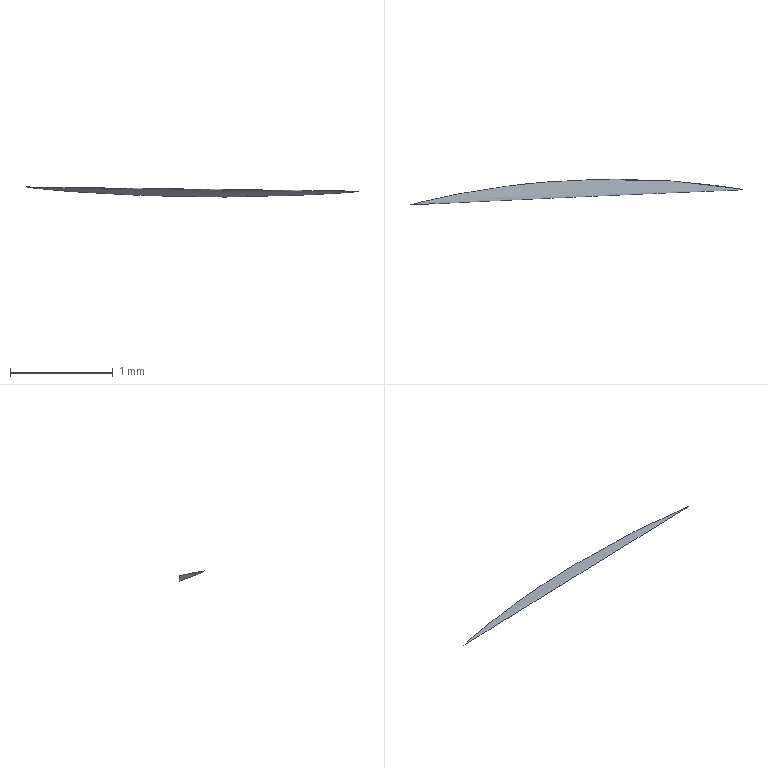Part | NX | features solid 2 | 1 solid | 2 faces | box 3.263 x 0.2526 x 0.09895 mm | volume 0.009083 mm3 | spline 1 | cylinder 1 | commonest cylinder face diameters 16 x1
STEP:
#1=CARTESIAN_POINT('',(196.075,-259.338,60.011));
#2=VERTEX_POINT('',#1);
#3=CARTESIAN_POINT('',(196.385,-259.369,60.026));
#4=CARTESIAN_POINT('',(195.693,-259.293,59.989));
#5=CARTESIAN_POINT('',(194.917,-259.297,59.986));
#6=CARTESIAN_POINT('',(194.063,-259.417,60.031));
#7=CARTESIAN_POINT('',(193.755,-259.475,60.051));
#8=CARTESIAN_POINT('',(193.469,-259.544,60.082));
#9=CARTESIAN_POINT('',(193.42,-259.557,60.087));
#10=CARTESIAN_POINT('',(193.407,-259.56,60.09));
#11=CARTESIAN_POINT('',(193.406,-259.56,60.091));
#12=CARTESIAN_POINT('',(193.405,-259.56,60.091));
#13=CARTESIAN_POINT('',(193.406,-259.56,60.091));
#14=CARTESIAN_POINT('',(193.407,-259.56,60.091));
#15=CARTESIAN_POINT('',(193.408,-259.559,60.092));
#16=CARTESIAN_POINT('',(193.418,-259.557,60.092));
#17=CARTESIAN_POINT('',(193.442,-259.551,60.092));
#18=CARTESIAN_POINT('',(193.501,-259.536,60.09));
#19=CARTESIAN_POINT('',(193.595,-259.513,60.086));
#20=CARTESIAN_POINT('',(193.891,-259.45,60.075));
#21=CARTESIAN_POINT('',(193.991,-259.433,60.07));
#22=CARTESIAN_POINT('',(194.358,-259.372,60.058));
#23=CARTESIAN_POINT('',(194.85,-259.32,60.047));
#24=CARTESIAN_POINT('',(195.597,-259.299,60.04));
#25=CARTESIAN_POINT('',(196.135,-259.333,60.043));
#26=CARTESIAN_POINT('',(196.605,-259.401,60.051));
#27=CARTESIAN_POINT('',(196.66,-259.41,60.051));
#28=CARTESIAN_POINT('',(196.667,-259.411,60.05));
#29=CARTESIAN_POINT('',(196.668,-259.411,60.05));
#30=CARTESIAN_POINT('',(196.669,-259.411,60.049));
#31=CARTESIAN_POINT('',(196.669,-259.411,60.049));
#32=CARTESIAN_POINT('',(196.668,-259.411,60.049));
#33=CARTESIAN_POINT('',(196.665,-259.411,60.048));
#34=CARTESIAN_POINT('',(196.654,-259.409,60.046));
#35=CARTESIAN_POINT('',(196.628,-259.405,60.044));
#36=CARTESIAN_POINT('',(196.57,-259.396,60.039));
#37=CARTESIAN_POINT('',(196.385,-259.369,60.026));
#38=CARTESIAN_POINT('',(195.693,-259.293,59.989));
#39=CARTESIAN_POINT('',(194.917,-259.297,59.986));
#40=B_SPLINE_CURVE_WITH_KNOTS('',3,(#3,#4,#5,#6,#7,#8,#9,#10,#11,#12,#13,#14,#15,#16,#17,#18,#19,#20,#21,#22,#23,#24,#25,#26,#27,#28,#29,#30,#31,#32,#33,#34,#35,#36,#37,#38,#39),.UNSPECIFIED.,.T.,.F.,(1,1,1,1,1,1,1,1,1,1,1,1,1,1,1,1,1,1,1,1,1,1,1,1,1,1,1,1,1,1,1,1,1,1,1,1,1,1,1,1,1),(-0.08614,-0.07853,-0.0633,0.,0.2375,0.3028,0.3681,0.4043,0.408,0.4091,0.4092,0.4092,0.4093,0.4094,0.4097,0.4101,0.4139,0.4215,0.4367,0.4668,0.4968,0.557,0.6171,0.7373,0.8681,0.9043,0.908,0.9084,0.9086,0.9086,0.9087,0.9087,0.9092,0.9101,0.9139,0.9215,0.9367,1.,1.238,1.303,1.368),.UNSPECIFIED.);
#41=EDGE_CURVE('',#2,#2,#40,.T.);
#42=ORIENTED_EDGE('',*,*,#41,.F.);
#43=EDGE_LOOP('',(#42));
#44=FACE_BOUND('',#43,.T.);
#45=CARTESIAN_POINT('',(201.017,-259.105,59.932));
#46=CARTESIAN_POINT('',(198.706,-259.154,59.95));
#47=CARTESIAN_POINT('',(196.396,-259.244,59.975));
#48=CARTESIAN_POINT('',(194.087,-259.349,60.002));
#49=CARTESIAN_POINT('',(200.711,-259.182,59.963));
#50=CARTESIAN_POINT('',(198.437,-259.233,59.981));
#51=CARTESIAN_POINT('',(196.163,-259.323,60.006));
#52=CARTESIAN_POINT('',(193.889,-259.43,60.034));
#53=CARTESIAN_POINT('',(200.06,-259.302,60.012));
#54=CARTESIAN_POINT('',(197.863,-259.358,60.031));
#55=CARTESIAN_POINT('',(195.666,-259.45,60.056));
#56=CARTESIAN_POINT('',(193.47,-259.557,60.085));
#57=CARTESIAN_POINT('',(198.711,-259.339,60.031));
#58=CARTESIAN_POINT('',(196.677,-259.403,60.052));
#59=CARTESIAN_POINT('',(194.644,-259.499,60.08));
#60=CARTESIAN_POINT('',(192.611,-259.608,60.109));
#61=CARTESIAN_POINT('',(197.132,-259.316,60.034));
#62=CARTESIAN_POINT('',(195.293,-259.369,60.052));
#63=CARTESIAN_POINT('',(193.453,-259.449,60.076));
#64=CARTESIAN_POINT('',(191.614,-259.54,60.101));
#65=CARTESIAN_POINT('',(195.896,-259.31,60.041));
#66=CARTESIAN_POINT('',(194.208,-259.355,60.057));
#67=CARTESIAN_POINT('',(192.52,-259.423,60.077));
#68=CARTESIAN_POINT('',(190.833,-259.501,60.099));
#69=CARTESIAN_POINT('',(195.349,-259.305,60.043));
#70=CARTESIAN_POINT('',(193.728,-259.347,60.058));
#71=CARTESIAN_POINT('',(192.108,-259.41,60.077));
#72=CARTESIAN_POINT('',(190.487,-259.482,60.097));
#73=B_SPLINE_SURFACE_WITH_KNOTS('',3,3,((#45,#46,#47,#48),(#49,#50,#51,#52),(#53,#54,#55,#56),(#57,#58,#59,#60),(#61,#62,#63,#64),(#65,#66,#67,#68),(#69,#70,#71,#72)),.UNSPECIFIED.,.F.,.F.,.F.,(4,1,1,1,4),(4,4),(0.2563,0.3125,0.375,0.5,0.5992),(0.08369,0.2274),.UNSPECIFIED.);
#74=ADVANCED_FACE('',(#44),#73,.T.);
#75=ORIENTED_EDGE('',*,*,#41,.T.);
#76=EDGE_LOOP('',(#75));
#77=FACE_BOUND('',#76,.T.);
#78=CARTESIAN_POINT('',(195.394,-267.309,230.));
#79=DIRECTION('',(0.,0.,-1.));
#80=DIRECTION('',(1.,0.,0.));
#81=AXIS2_PLACEMENT_3D('',#78,#79,#80);
#82=CYLINDRICAL_SURFACE('',#81,8.);
#83=ADVANCED_FACE('',(#77),#82,.T.);
#84=CLOSED_SHELL('',(#74,#83));
#85=MANIFOLD_SOLID_BREP('',#84);
#86=(LENGTH_UNIT()NAMED_UNIT(*)SI_UNIT(.MILLI.,.METRE.));
#87=UNCERTAINTY_MEASURE_WITH_UNIT(LENGTH_MEASURE(0.0508),#86,'','');
#88=(NAMED_UNIT(*)PLANE_ANGLE_UNIT()SI_UNIT($,.RADIAN.));
#89=(NAMED_UNIT(*)SI_UNIT($,.STERADIAN.)SOLID_ANGLE_UNIT());
#90=(GEOMETRIC_REPRESENTATION_CONTEXT(3)GLOBAL_UNCERTAINTY_ASSIGNED_CONTEXT((#87))GLOBAL_UNIT_ASSIGNED_CONTEXT((#86,#88,#89))REPRESENTATION_CONTEXT('',''));
#91=ADVANCED_BREP_SHAPE_REPRESENTATION('',(#85),#90);